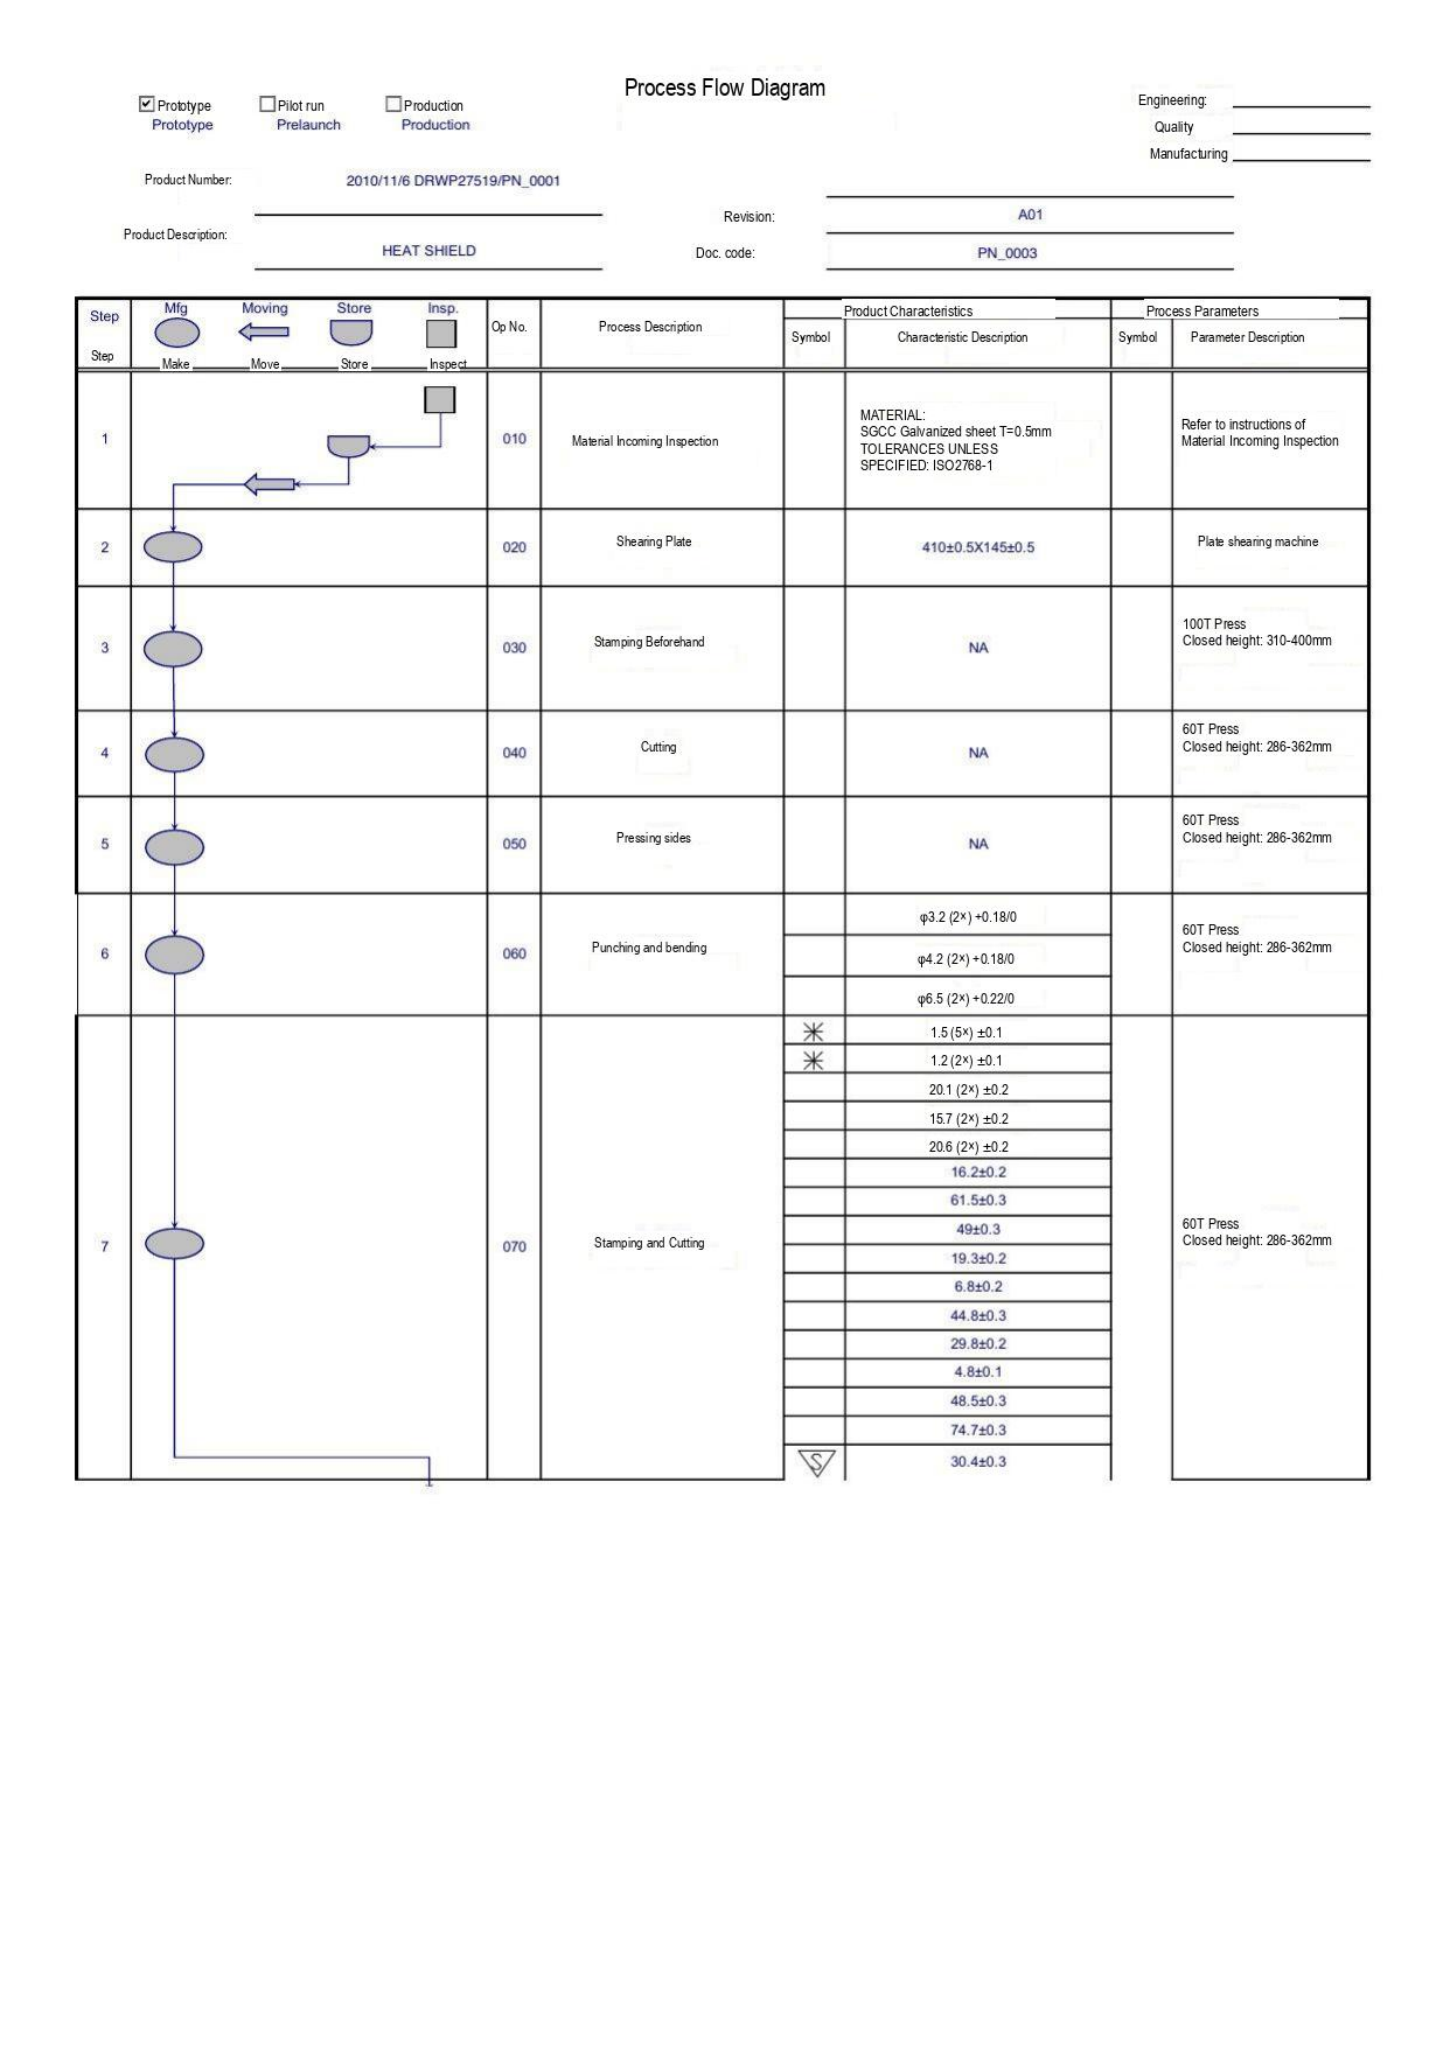# Process Flow Diagram

☑ Prototype
Prototype

☐ Pilot run
Prelaunch

☐ Production
Production

Engineering: 
Quality 
Manufacturing 

Product Number: 2010/11/6 DRWP27519/PN_0001

Product Description: HEAT SHIELD

Revision: A01

Doc. code: PN_0003

| Step<br>Step | Mfg Make / Moving Move / Store Store / Insp. Inspect | Op No. | Process Description | Product Characteristics<br>Symbol | Product Characteristics<br>Characteristic Description | Process Parameters<br>Symbol | Process Parameters<br>Parameter Description |
|---|---|---|---|---|---|---|---|
| 1 | | 010 | Material Incoming Inspection | | MATERIAL:<br>SGCC Galvanized sheet T=0.5mm<br>TOLERANCES UNLESS<br>SPECIFIED: ISO2768-1 | | Refer to instructions of Material Incoming Inspection |
| 2 | | 020 | Shearing Plate | | 410±0.5X145±0.5 | | Plate shearing machine |
| 3 | | 030 | Stamping Beforehand | | NA | | 100T Press<br>Closed height: 310-400mm |
| 4 | | 040 | Cutting | | NA | | 60T Press<br>Closed height: 286-362mm |
| 5 | | 050 | Pressing sides | | NA | | 60T Press<br>Closed height: 286-362mm |
| 6 | | 060 | Punching and bending | | φ3.2 (2×) +0.18/0 | | 60T Press<br>Closed height: 286-362mm |
| | | | | | φ4.2 (2×) +0.18/0 | | |
| | | | | | φ6.5 (2×) +0.22/0 | | |
| 7 | | 070 | Stamping and Cutting | ✳ | 1.5 (5×) ±0.1 | | 60T Press<br>Closed height: 286-362mm |
| | | | | ✳ | 1.2 (2×) ±0.1 | | |
| | | | | | 20.1 (2×) ±0.2 | | |
| | | | | | 15.7 (2×) ±0.2 | | |
| | | | | | 20.6 (2×) ±0.2 | | |
| | | | | | 16.2±0.2 | | |
| | | | | | 61.5±0.3 | | |
| | | | | | 49±0.3 | | |
| | | | | | 19.3±0.2 | | |
| | | | | | 6.8±0.2 | | |
| | | | | | 44.8±0.3 | | |
| | | | | | 29.8±0.2 | | |
| | | | | | 4.8±0.1 | | |
| | | | | | 48.5±0.3 | | |
| | | | | | 74.7±0.3 | | |
| | | | | S | 30.4±0.3 | | |
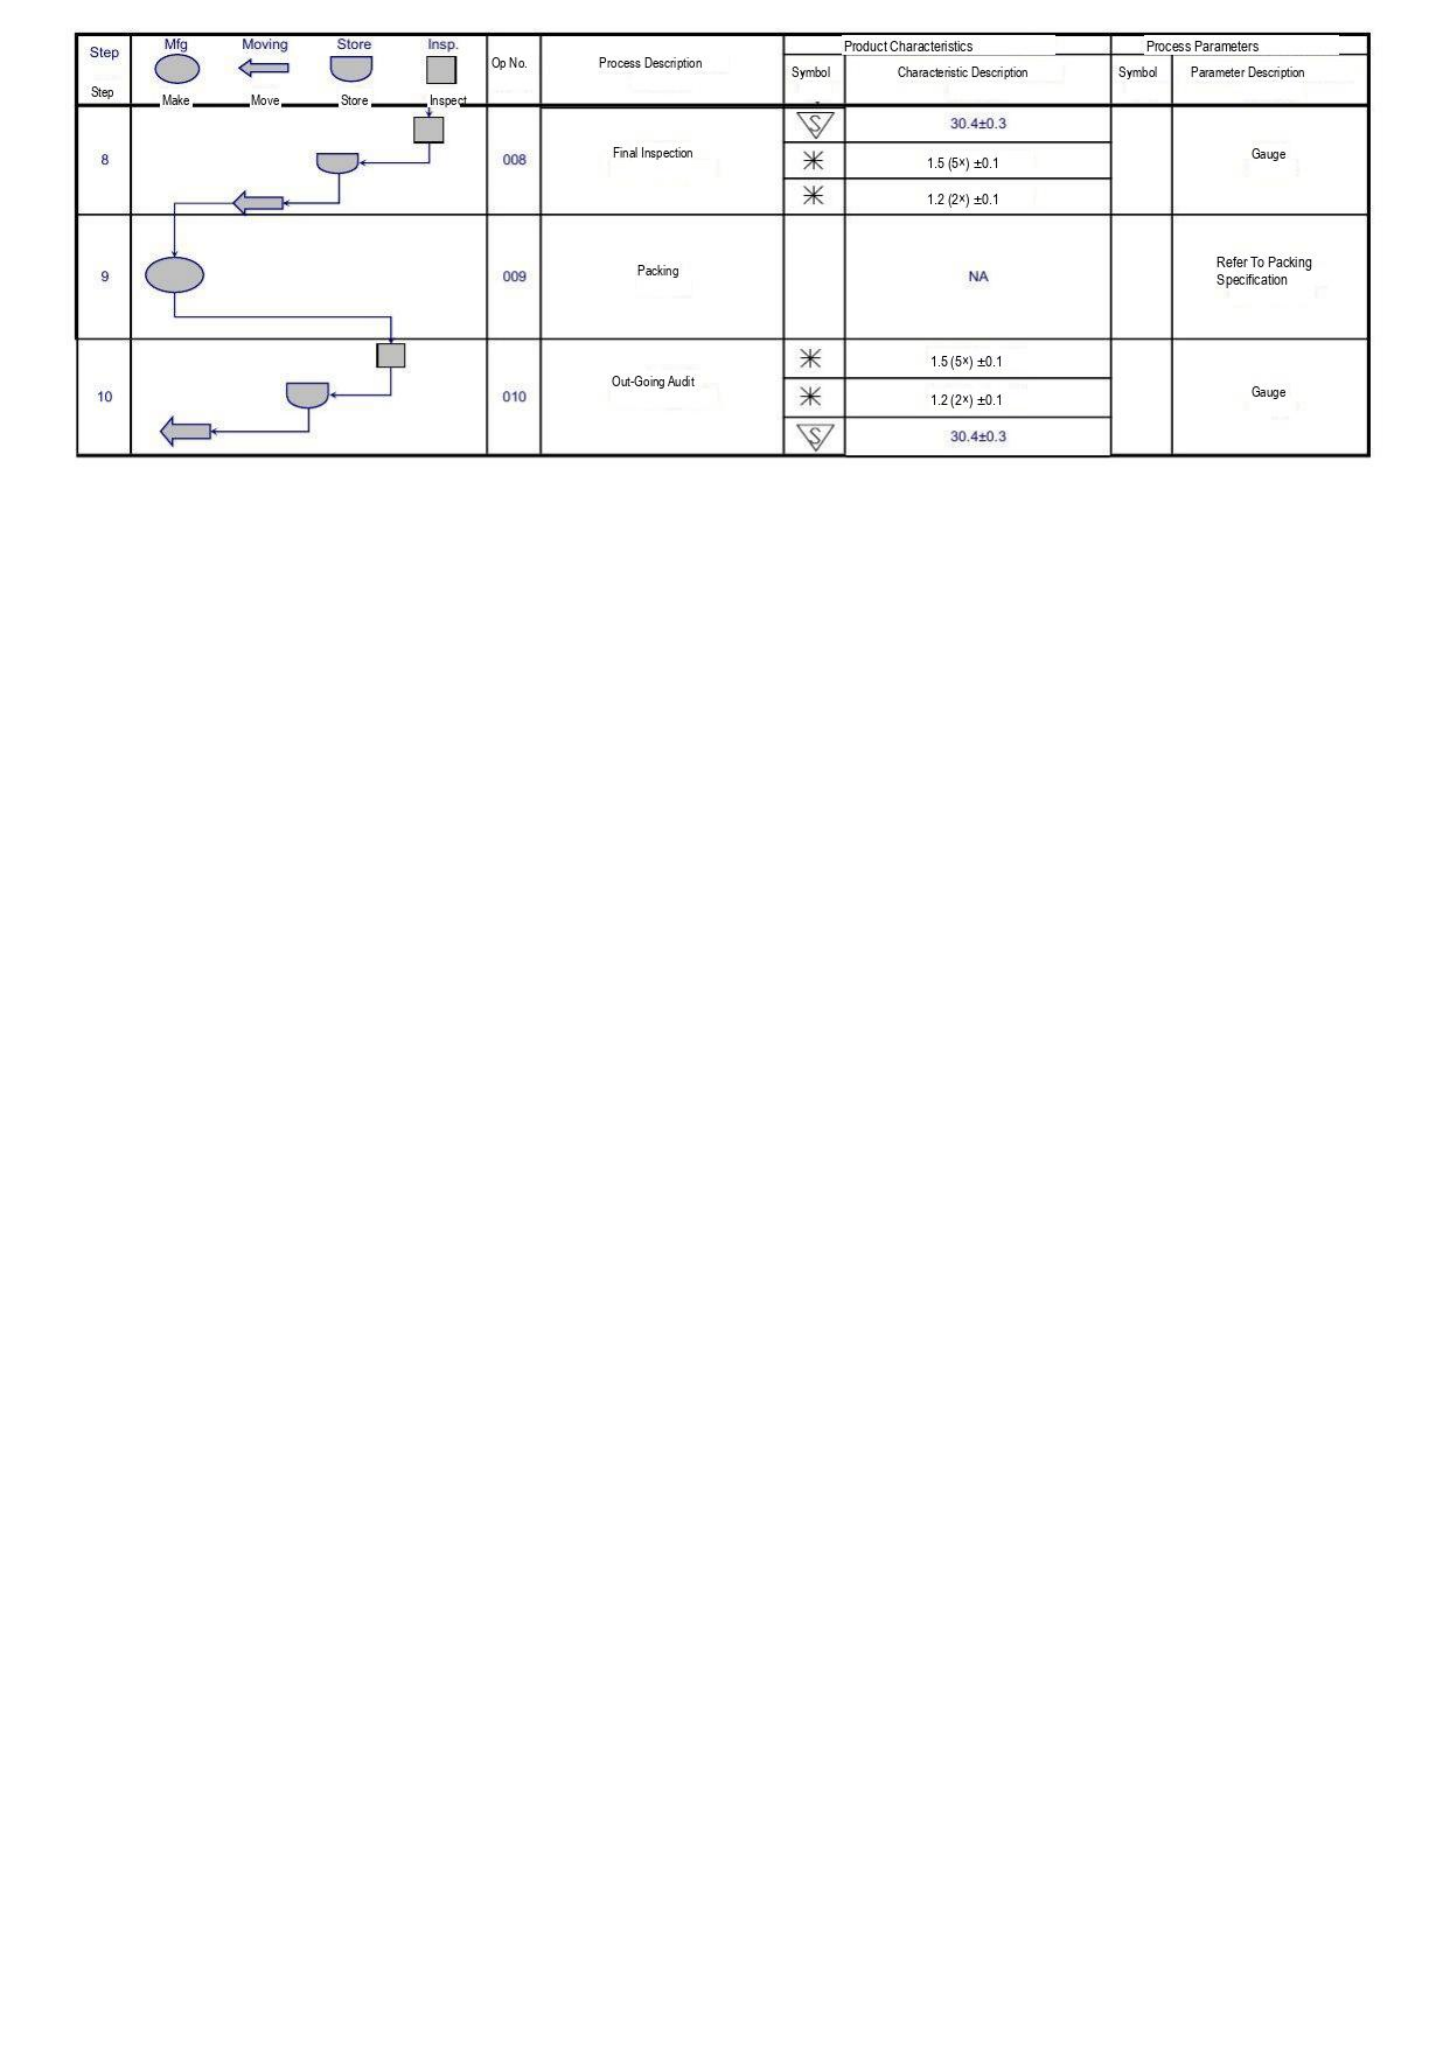| Step<br>Step | Mfg<br>Make | Moving<br>Move | Store<br>Store | Insp.<br>Inspect | Op No. | Process Description | Product Characteristics<br>Symbol | Product Characteristics<br>Characteristic Description | Process Parameters<br>Symbol | Process Parameters<br>Parameter Description |
|---|---|---|---|---|---|---|---|---|---|---|
| 8 | | | | | 008 | Final Inspection | S | 30.4±0.3 | | Gauge |
| | | | | | | | | 1.5 (5×) ±0.1 | | |
| | | | | | | | | 1.2 (2×) ±0.1 | | |
| 9 | | | | | 009 | Packing | | NA | | Refer To Packing Specification |
| 10 | | | | | 010 | Out-Going Audit | | 1.5 (5×) ±0.1 | | Gauge |
| | | | | | | | | 1.2 (2×) ±0.1 | | |
| | | | | | | | S | 30.4±0.3 | | |